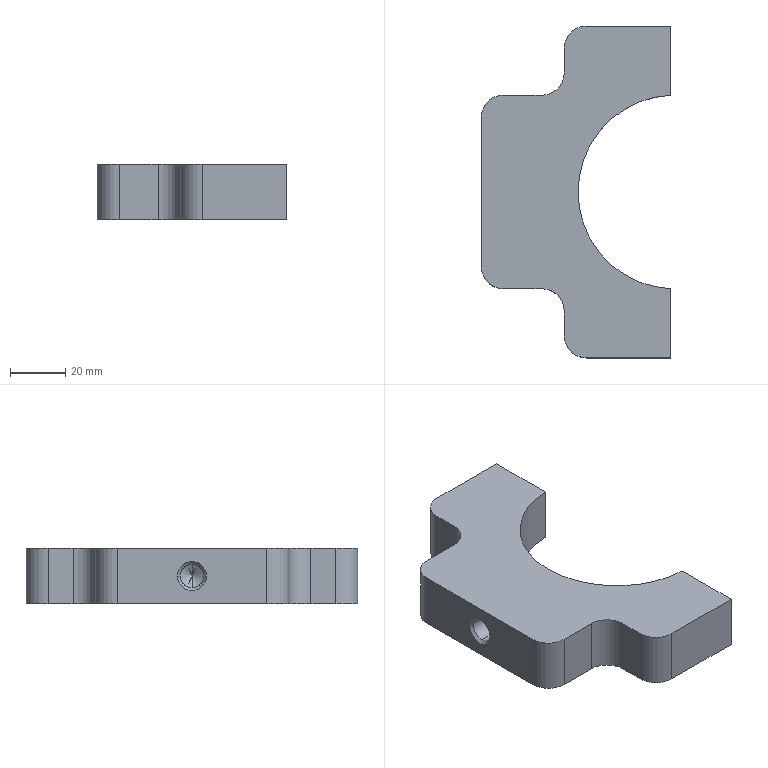Part | STEP file | Handle seat new 1 | 1 solid | 48 faces | box 68.5 x 120 x 20 mm | volume 85047 mm3 | cylinder 24 | plane 20 | cone 4 | commonest cylinder face diameters 16 x6 4 x4 6.8 x4 8 x4 8.5 x2 12 x2